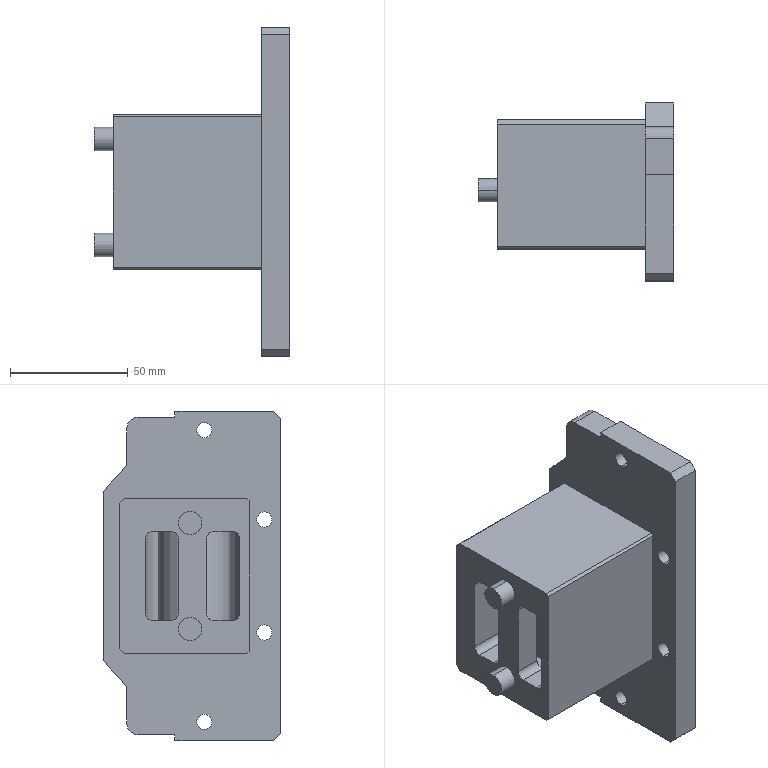Part | NX | features BREP 5 | 5 solids | 122 faces | box 83 x 75.5 x 140 mm | volume 294891 mm3 | cylinder 66 | plane 48 | cone 8 | commonest cylinder face diameters 6 x12 10 x10 6.5 x8 11 x8 3 x4 3.3 x4